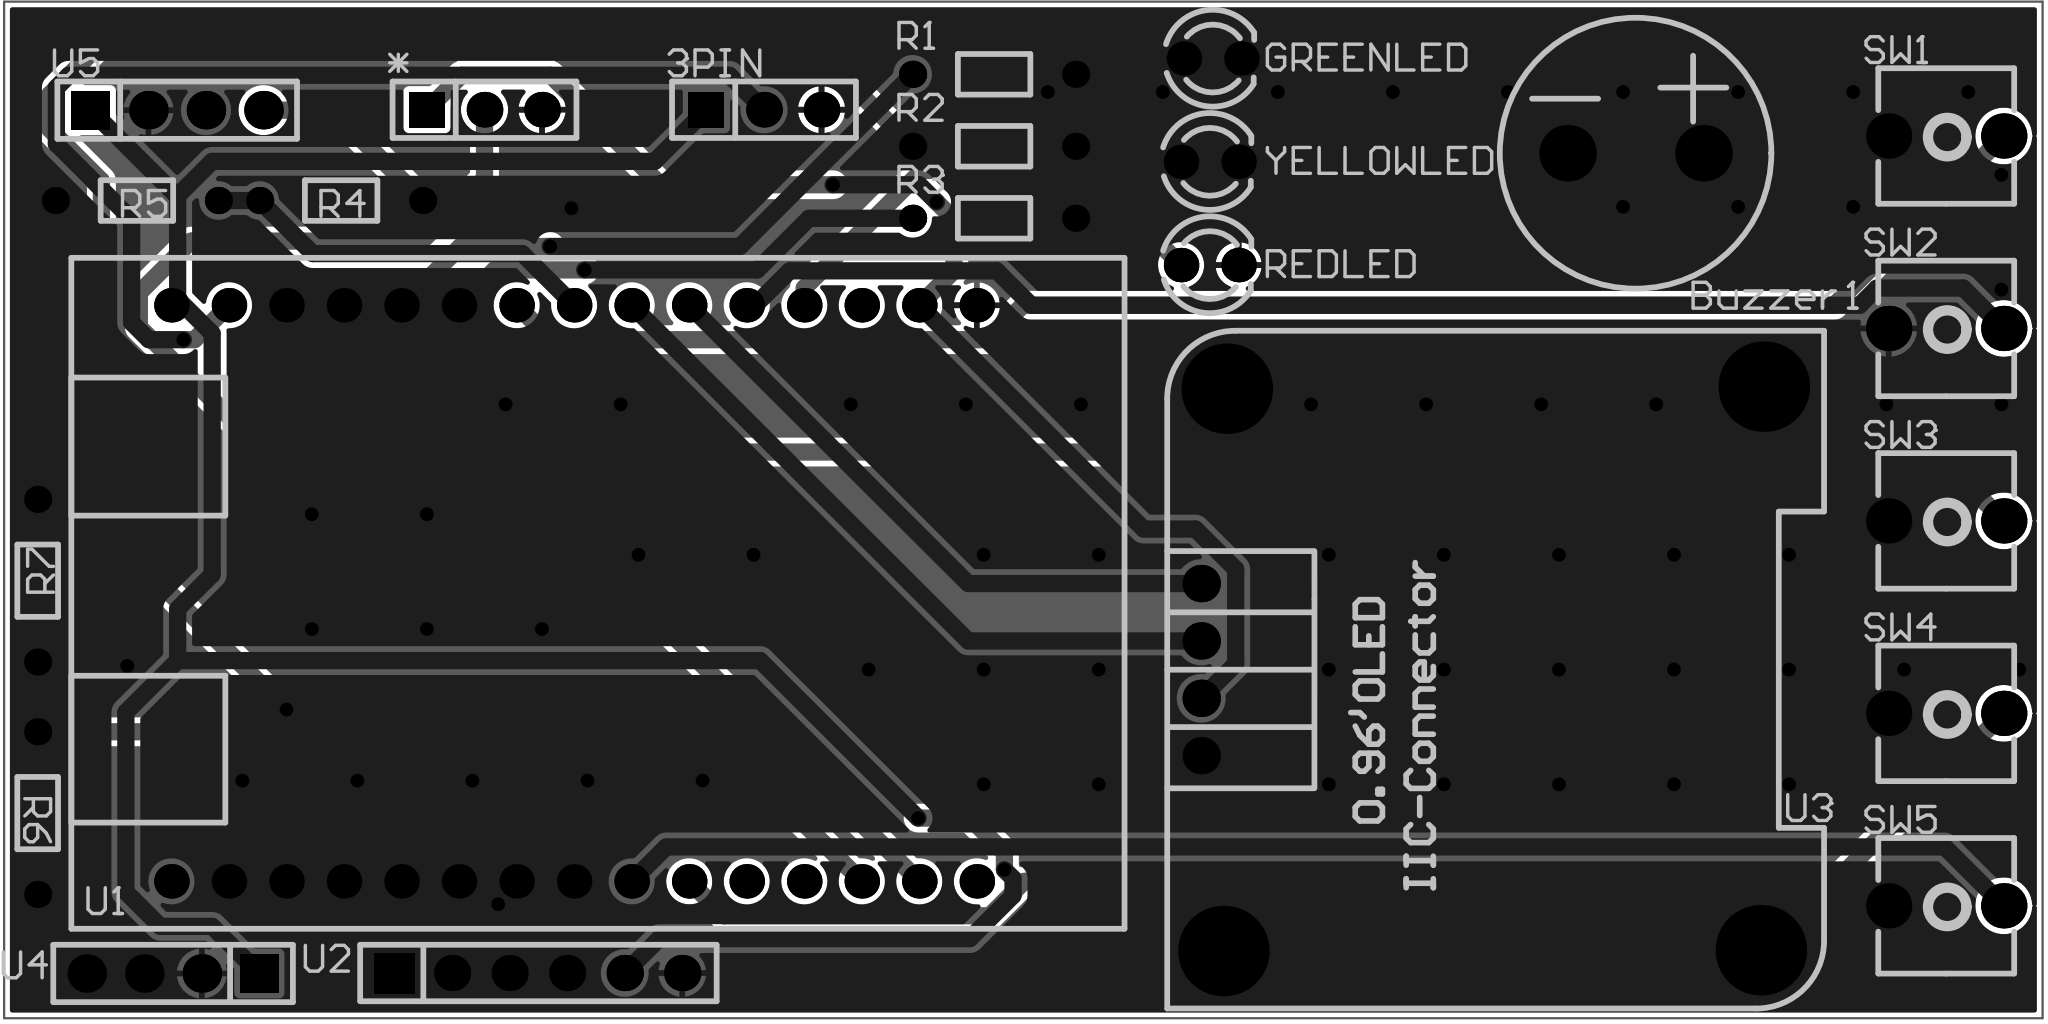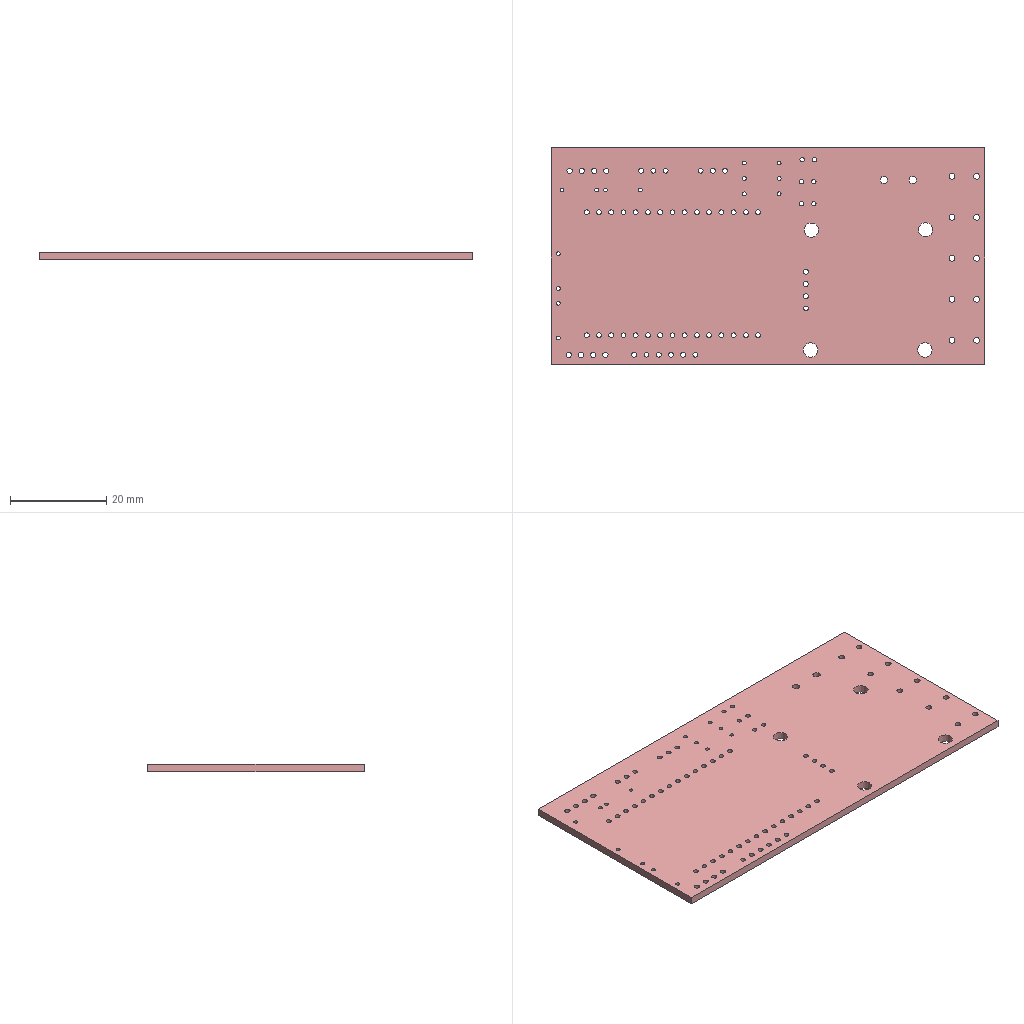Circuit board layout | Altium Designer | box 90 x 45 x 1.6 mm
Layer stack:
# Altium Designer layer stack of  (unit mm; dielectric type: 0 none, 1 core, 2 prepreg, 3 surface material)
index,name,kind,layer,copper_thickness_mm,dielectric_type,dielectric_thickness_mm,dielectric_material,dielectric_constant
0,Top Paste Mask Layer,other,,,,,,
1,Top Silkscreen Layer,other,,,,,,
2,Top Solder Mask Layer,dielectric,,,3,0.01,,3.3
3,Top Layer,copper,Top Layer,0.035,,,,
4,Dielectric1,dielectric,,,3,1.51,FR4,4.5
5,Bottom Layer,copper,Bottom Layer,0.035,,,,
6,Bottom Solder Mask Layer,dielectric,,,3,0.01,,3.3
7,Bottom Silkscreen Layer,other,,,,,,
8,Bottom Paste Mask Layer,other,,,,,,
# drill layer pairs: low layer,high layer
drill_pair,Top Layer,Bottom Layer
Part placement:
Designator,Comment,Layer,Footprint,Center-X(mm),Center-Y(mm),Rotation
3PIN,,TopLayer,HDR-TH_3P-P2.54-V-F,115.443,121.178,0
*,DHT11,TopLayer,HDR-TH_3P-P2.54-V-F,103.104,121.178,0
Buzzer1,Buzzer,TopLayer,BUZ-TH_BD12.0-P6.00-D0.9-RD,153.924,119.253,0
GREENLED,LED_3M,TopLayer,LED_TH-3mm,135.255,123.444,0
R1,220,TopLayer,Res_1/8W,125.603,122.745,0
R2,220,TopLayer,Res_1/8W,125.603,119.559,0
R3,220,TopLayer,Res_1/8W,125.603,116.373,0
REDLED,LED_3M,TopLayer,LED_TH-3mm,135.128,114.3,0
SW1,SELECT,TopLayer,KEY-TH_2P-L6.0-W6.0-P5.00,167.64,120.015,0
SW2,CONFIRM,TopLayer,KEY-TH_2P-L6.0-W6.0-P5.00,167.64,111.496,0
SW3,INCREASE,TopLayer,KEY-TH_2P-L6.0-W6.0-P5.00,167.64,102.977,0
SW4,DECREASE,TopLayer,KEY-TH_2P-L6.0-W6.0-P5.00,167.64,94.458,0
SW5,Off,TopLayer,KEY-TH_2P-L6.0-W6.0-P5.00,167.64,85.939,0
U1,ESP32-C6,TopLayer,HDR-TH_33P-P2.54-V-R2-C15-S2.54_C9041,107.061,99.772,180
U2,MicroSD,TopLayer,HDR-TH_6P-P2.54-V-F,105.483,82.964,0
U3,OLED_SSD1306,TopLayer,0.96OLED_4P,147.166,96.428,90
U4,MQ7,TopLayer,HDR-TH_4P-P2.54-V-F,89.354,82.944,180
U5,MQ135,TopLayer,HDR-TH_4P-P2.54-V-F,89.535,121.158,0
YELLOWLED,LED_3M,TopLayer,LED_TH-3mm,135.128,118.872,0
R4,15kΩ,TopLayer,Res_1/8W,96.774,117.158,180
R5,27kΩ,TopLayer,Res_1/8W,87.757,117.158,180
R6,15kΩ,TopLayer,Res_1/8W,83.375,90.043,270
R7,27kΩ,TopLayer,Res_1/8W,83.376,100.33,90
Pad and via stacks:
# Altium Designer via and pad stacks of  (unit mm). Each distinct definition once, with the count of objects using it.
# via: kind,start_layer,end_layer,hole_mm,diameter_mm,mode(0 simple;1 top-mid-bottom;2 full stack),diameter_per_layer,count,example_net
# pad: kind,layer,hole_mm,hole_type(0 round;1 square;2 slot),plating,top_size,top_shape(1 round;2 rect;3 octagon;9 rounded rect),mid_size,bottom_size,mode,footprint,size_per_layer,count,example
pad,Multi-Layer,1.02,0,plated,1.575x1.575,1,1.575x1.575,1.575x1.575,0,HDR-TH_3P-P2.54-V-F,,4,3PIN.3
pad,Multi-Layer,1.02,0,plated,1.575x1.575,2,1.575x1.575,1.575x1.575,0,HDR-TH_3P-P2.54-V-F,,2,3PIN.1
pad,Multi-Layer,1.5,0,plated,2.5x2.5,1,2.5x2.5,2.5x2.5,0,BUZ-TH_BD12.0-P6.00-D0.9-RD,,2,Buzzer1.1
pad,Multi-Layer,0.9144,0,plated,1.524x1.524,1,1.524x1.524,1.524x1.524,0,LED_TH-3mm,,6,GREENLED.1
pad,Multi-Layer,0.8001,0,plated,1.199x1.199,1,1.199x1.199,1.199x1.199,0,Res_1/8W,,14,R1.1
pad,Multi-Layer,1.2,0,plated,2x2,1,2x2,2x2,0,KEY-TH_2P-L6.0-W6.0-P5.00,,10,SW1.2
pad,Multi-Layer,1,0,plated,1.524x1.524,1,1.524x1.524,1.524x1.524,0,HDR-TH_33P-P2.54-V-R2-C15-S2.54_C9041,,30,U1.1
pad,Multi-Layer,1.02,0,plated,1.6x1.6,1,1.6x1.6,1.6x1.6,0,HDR-TH_6P-P2.54-V-F,,5,U2.6
pad,Multi-Layer,1.02,0,plated,1.8x1.8,2,1.8x1.8,1.8x1.8,0,HDR-TH_6P-P2.54-V-F,,1,U2.1
pad,Multi-Layer,3,0,plated,4x4,1,4x4,4x4,0,0.96OLED_4P,,4,U3.5
pad,Multi-Layer,1,0,plated,1.65x1.65,1,1.65x1.65,1.65x1.65,0,0.96OLED_4P,,4,U3.4
pad,Multi-Layer,1.1,0,plated,1.7x1.7,2,1.7x1.7,1.7x1.7,0,HDR-TH_4P-P2.54-V-F,,2,U4.1
pad,Multi-Layer,1.1,0,plated,1.7x1.7,1,1.7x1.7,1.7x1.7,0,HDR-TH_4P-P2.54-V-F,,6,U4.2
via,Top Layer,Bottom Layer,0.3048,0.61,0,,72,$1N15
Copper pours:
name,layer,net,type(0 solid;1 hatched;2 none)
Top Layer-GND,Top Layer,GND,0
Bottom Layer-GND,Bottom Layer,GND,0
Design rules, without the lines most boards share:
# Altium Designer design rules of  (exported by Altium Designer, unit mm)
# columns: name | kind | enabled | priority | scope1 | scope2 | descriptor | typed fields (field=value)
copperThickness1oz_2 | 2 | enabled | 2 | All | All | Width Constraint (Min=5mil) (Max=100mil) (Preferred=30mil) (All) |
viaSize | 11 | enabled | 1 | All | All | Routing Via (MinHoleWidth=11.811mil) (MaxHoleWidth=248.032mil) (PreferredHoleWidth=12.008mil) (MinWidth=19.685mil) (MaxWidth=393.701mil) (PreferedWidth=24.016mil) (All) | via_min_hole=0.3 via_max_hole=6.3 via_preferred_diameter=0.61 via_preferred_hole=0.305
solderMaskExpansion | 13 | enabled | 2 | All | All | Solder Mask Expansion (Expansion =2.008mil) (All) | expansion=0.051